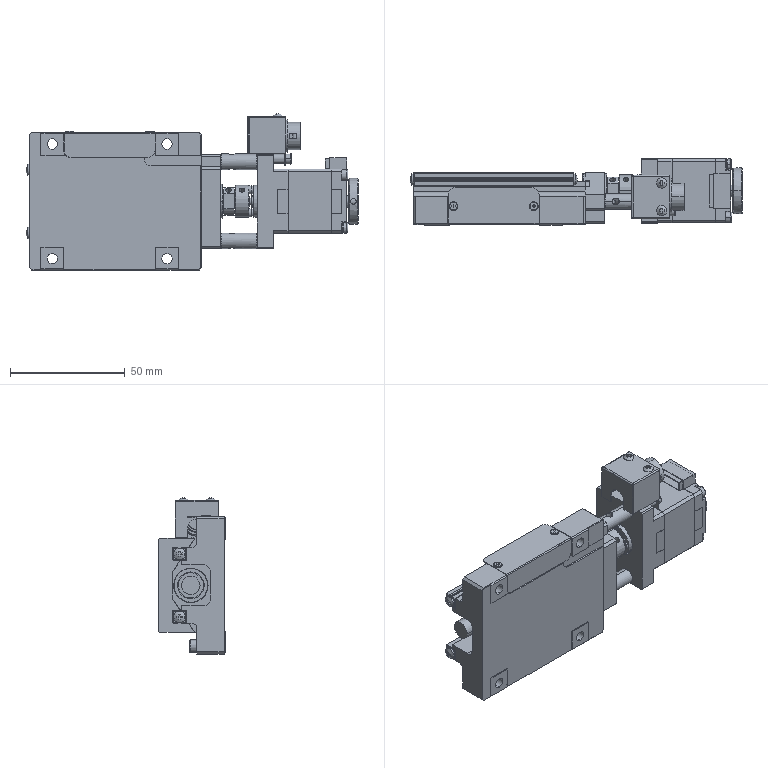Part | SolidWorks | features BaseBody 23 | 23 solids | 1525 faces | box 144.767 x 29 x 68.134 mm | volume 103226 mm3 | plane 918 | cylinder 420 | cone 99 | spline 46 | torus 42 | commonest cylinder face diameters 4.5 x46 2.5 x26 0.6 x24 3.8 x20 10.5 x17 8 x16